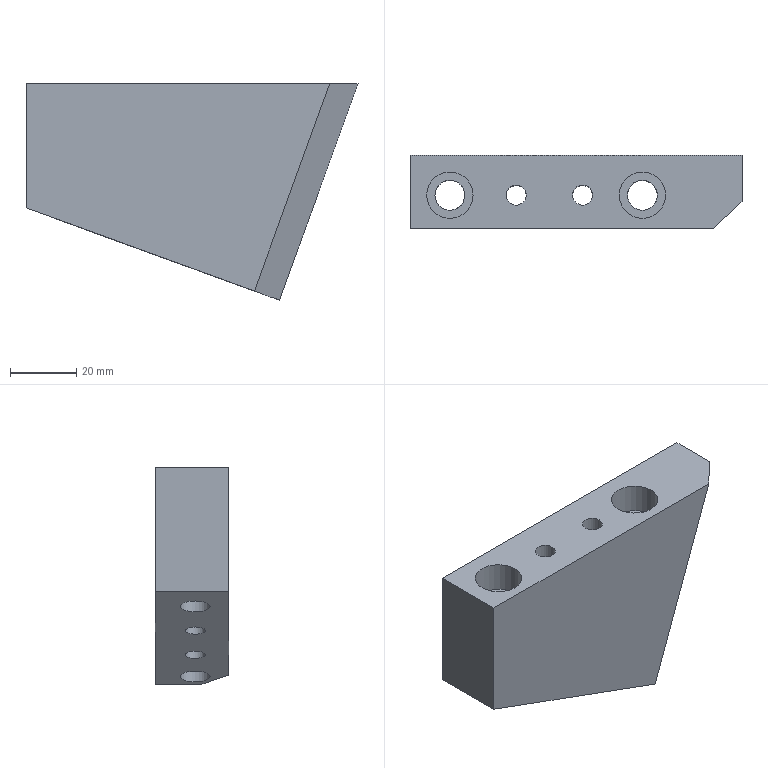Part | STEP file | P011002S002-005 | 1 solid | 15 faces | box 100 x 22 x 65.128 mm | volume 89552 mm3 | plane 9 | cylinder 6 | commonest cylinder face diameters 6 x2 9 x2 14 x2
STEP:
#1=CARTESIAN_POINT('',(0.,0.,0.));
#2=DIRECTION('',(0.,0.,1.));
#3=DIRECTION('',(1.,0.,0.));
#4=AXIS2_PLACEMENT_3D('',#1,#2,#3);
#5=CARTESIAN_POINT('',(194.,-102.,19.));
#6=VERTEX_POINT('',#5);
#7=CARTESIAN_POINT('',(200.,-102.,19.));
#8=VERTEX_POINT('',#7);
#9=CARTESIAN_POINT('',(197.,-102.,19.));
#10=DIRECTION('',(0.,0.,-1.));
#11=DIRECTION('',(-1.,0.,0.));
#12=AXIS2_PLACEMENT_3D('',#9,#10,#11);
#13=CIRCLE('',#12,3.);
#14=CARTESIAN_POINT('',(-275.,-277.,19.));
#15=DIRECTION('',(0.,0.,1.));
#16=DIRECTION('',(-1.,0.,0.));
#17=AXIS2_PLACEMENT_3D('',#14,#15,#16);
#18=PLANE('',#17);
#19=CARTESIAN_POINT('',(-469.,-175.));
#20=CARTESIAN_POINT('',(-469.,-180.196));
#21=CARTESIAN_POINT('',(-473.5,-177.598));
#22=CARTESIAN_POINT('',(-478.,-175.));
#23=CARTESIAN_POINT('',(-473.5,-172.402));
#24=CARTESIAN_POINT('',(-469.,-169.804));
#25=CARTESIAN_POINT('',(-469.,-175.));
#26=(BOUNDED_CURVE()B_SPLINE_CURVE(2,(#19,#20,#21,#22,#23,#24,#25),.UNSPECIFIED.,.T.,.F.)B_SPLINE_CURVE_WITH_KNOTS((1,2,2,2,2,1),(-2.094,0.,2.094,4.189,6.283,8.378),.UNSPECIFIED.)CURVE()GEOMETRIC_REPRESENTATION_ITEM()RATIONAL_B_SPLINE_CURVE((1.,0.5,1.,0.5,1.,0.5,1.))REPRESENTATION_ITEM(''));
#27=(GEOMETRIC_REPRESENTATION_CONTEXT(2)PARAMETRIC_REPRESENTATION_CONTEXT()REPRESENTATION_CONTEXT('',''));
#28=DEFINITIONAL_REPRESENTATION('',(#26),#27);
#29=PCURVE('',#18,#28);
#30=CARTESIAN_POINT('',(197.,-102.,19.));
#31=DIRECTION('',(0.,0.,-1.));
#32=DIRECTION('',(1.,0.,0.));
#33=AXIS2_PLACEMENT_3D('',#30,#31,#32);
#34=CYLINDRICAL_SURFACE('',#33,3.);
#35=CARTESIAN_POINT('',(3.142,0.));
#36=DIRECTION('',(1.,0.));
#37=VECTOR('',#36,1.);
#38=LINE('',#35,#37);
#39=(GEOMETRIC_REPRESENTATION_CONTEXT(2)PARAMETRIC_REPRESENTATION_CONTEXT()REPRESENTATION_CONTEXT('',''));
#40=DEFINITIONAL_REPRESENTATION('',(#38),#39);
#41=PCURVE('',#34,#40);
#42=SURFACE_CURVE('',#13,(#29,#41),.PCURVE_S1.);
#43=EDGE_CURVE('',#6,#8,#42,.T.);
#44=ORIENTED_EDGE('',*,*,#43,.T.);
#45=CARTESIAN_POINT('',(197.,-102.,19.));
#46=DIRECTION('',(0.,0.,-1.));
#47=DIRECTION('',(-1.,0.,0.));
#48=AXIS2_PLACEMENT_3D('',#45,#46,#47);
#49=CIRCLE('',#48,3.);
#50=CARTESIAN_POINT('',(-469.,-175.));
#51=CARTESIAN_POINT('',(-469.,-180.196));
#52=CARTESIAN_POINT('',(-473.5,-177.598));
#53=CARTESIAN_POINT('',(-478.,-175.));
#54=CARTESIAN_POINT('',(-473.5,-172.402));
#55=CARTESIAN_POINT('',(-469.,-169.804));
#56=CARTESIAN_POINT('',(-469.,-175.));
#57=(BOUNDED_CURVE()B_SPLINE_CURVE(2,(#50,#51,#52,#53,#54,#55,#56),.UNSPECIFIED.,.T.,.F.)B_SPLINE_CURVE_WITH_KNOTS((1,2,2,2,2,1),(-2.094,0.,2.094,4.189,6.283,8.378),.UNSPECIFIED.)CURVE()GEOMETRIC_REPRESENTATION_ITEM()RATIONAL_B_SPLINE_CURVE((1.,0.5,1.,0.5,1.,0.5,1.))REPRESENTATION_ITEM(''));
#58=(GEOMETRIC_REPRESENTATION_CONTEXT(2)PARAMETRIC_REPRESENTATION_CONTEXT()REPRESENTATION_CONTEXT('',''));
#59=DEFINITIONAL_REPRESENTATION('',(#57),#58);
#60=PCURVE('',#18,#59);
#61=CARTESIAN_POINT('',(-3.142,0.));
#62=DIRECTION('',(1.,0.));
#63=VECTOR('',#62,1.);
#64=LINE('',#61,#63);
#65=(GEOMETRIC_REPRESENTATION_CONTEXT(2)PARAMETRIC_REPRESENTATION_CONTEXT()REPRESENTATION_CONTEXT('',''));
#66=DEFINITIONAL_REPRESENTATION('',(#64),#65);
#67=PCURVE('',#34,#66);
#68=SURFACE_CURVE('',#49,(#60,#67),.PCURVE_S1.);
#69=EDGE_CURVE('',#8,#6,#68,.T.);
#70=ORIENTED_EDGE('',*,*,#69,.T.);
#71=EDGE_LOOP('',(#44,#70));
#72=FACE_BOUND('',#71,.T.);
#73=CARTESIAN_POINT('',(214.,-102.,19.));
#74=VERTEX_POINT('',#73);
#75=CARTESIAN_POINT('',(220.,-102.,19.));
#76=VERTEX_POINT('',#75);
#77=CARTESIAN_POINT('',(217.,-102.,19.));
#78=DIRECTION('',(0.,0.,-1.));
#79=DIRECTION('',(-1.,0.,0.));
#80=AXIS2_PLACEMENT_3D('',#77,#78,#79);
#81=CIRCLE('',#80,3.);
#82=CARTESIAN_POINT('',(-489.,-175.));
#83=CARTESIAN_POINT('',(-489.,-180.196));
#84=CARTESIAN_POINT('',(-493.5,-177.598));
#85=CARTESIAN_POINT('',(-498.,-175.));
#86=CARTESIAN_POINT('',(-493.5,-172.402));
#87=CARTESIAN_POINT('',(-489.,-169.804));
#88=CARTESIAN_POINT('',(-489.,-175.));
#89=(BOUNDED_CURVE()B_SPLINE_CURVE(2,(#82,#83,#84,#85,#86,#87,#88),.UNSPECIFIED.,.T.,.F.)B_SPLINE_CURVE_WITH_KNOTS((1,2,2,2,2,1),(-2.094,0.,2.094,4.189,6.283,8.378),.UNSPECIFIED.)CURVE()GEOMETRIC_REPRESENTATION_ITEM()RATIONAL_B_SPLINE_CURVE((1.,0.5,1.,0.5,1.,0.5,1.))REPRESENTATION_ITEM(''));
#90=(GEOMETRIC_REPRESENTATION_CONTEXT(2)PARAMETRIC_REPRESENTATION_CONTEXT()REPRESENTATION_CONTEXT('',''));
#91=DEFINITIONAL_REPRESENTATION('',(#89),#90);
#92=PCURVE('',#18,#91);
#93=CARTESIAN_POINT('',(217.,-102.,19.));
#94=DIRECTION('',(0.,0.,-1.));
#95=DIRECTION('',(1.,0.,0.));
#96=AXIS2_PLACEMENT_3D('',#93,#94,#95);
#97=CYLINDRICAL_SURFACE('',#96,3.);
#98=CARTESIAN_POINT('',(3.142,0.));
#99=DIRECTION('',(1.,0.));
#100=VECTOR('',#99,1.);
#101=LINE('',#98,#100);
#102=(GEOMETRIC_REPRESENTATION_CONTEXT(2)PARAMETRIC_REPRESENTATION_CONTEXT()REPRESENTATION_CONTEXT('',''));
#103=DEFINITIONAL_REPRESENTATION('',(#101),#102);
#104=PCURVE('',#97,#103);
#105=SURFACE_CURVE('',#81,(#92,#104),.PCURVE_S1.);
#106=EDGE_CURVE('',#74,#76,#105,.T.);
#107=ORIENTED_EDGE('',*,*,#106,.T.);
#108=CARTESIAN_POINT('',(217.,-102.,19.));
#109=DIRECTION('',(0.,0.,-1.));
#110=DIRECTION('',(-1.,0.,0.));
#111=AXIS2_PLACEMENT_3D('',#108,#109,#110);
#112=CIRCLE('',#111,3.);
#113=CARTESIAN_POINT('',(-489.,-175.));
#114=CARTESIAN_POINT('',(-489.,-180.196));
#115=CARTESIAN_POINT('',(-493.5,-177.598));
#116=CARTESIAN_POINT('',(-498.,-175.));
#117=CARTESIAN_POINT('',(-493.5,-172.402));
#118=CARTESIAN_POINT('',(-489.,-169.804));
#119=CARTESIAN_POINT('',(-489.,-175.));
#120=(BOUNDED_CURVE()B_SPLINE_CURVE(2,(#113,#114,#115,#116,#117,#118,#119),.UNSPECIFIED.,.T.,.F.)B_SPLINE_CURVE_WITH_KNOTS((1,2,2,2,2,1),(-2.094,0.,2.094,4.189,6.283,8.378),.UNSPECIFIED.)CURVE()GEOMETRIC_REPRESENTATION_ITEM()RATIONAL_B_SPLINE_CURVE((1.,0.5,1.,0.5,1.,0.5,1.))REPRESENTATION_ITEM(''));
#121=(GEOMETRIC_REPRESENTATION_CONTEXT(2)PARAMETRIC_REPRESENTATION_CONTEXT()REPRESENTATION_CONTEXT('',''));
#122=DEFINITIONAL_REPRESENTATION('',(#120),#121);
#123=PCURVE('',#18,#122);
#124=CARTESIAN_POINT('',(-3.142,0.));
#125=DIRECTION('',(1.,0.));
#126=VECTOR('',#125,1.);
#127=LINE('',#124,#126);
#128=(GEOMETRIC_REPRESENTATION_CONTEXT(2)PARAMETRIC_REPRESENTATION_CONTEXT()REPRESENTATION_CONTEXT('',''));
#129=DEFINITIONAL_REPRESENTATION('',(#127),#128);
#130=PCURVE('',#97,#129);
#131=SURFACE_CURVE('',#112,(#123,#130),.PCURVE_S1.);
#132=EDGE_CURVE('',#76,#74,#131,.T.);
#133=ORIENTED_EDGE('',*,*,#132,.T.);
#134=EDGE_LOOP('',(#107,#133));
#135=FACE_BOUND('',#134,.T.);
#136=CARTESIAN_POINT('',(265.,-90.,19.));
#137=VERTEX_POINT('',#136);
#138=CARTESIAN_POINT('',(265.,-104.,19.));
#139=VERTEX_POINT('',#138);
#140=CARTESIAN_POINT('',(265.,30.,19.));
#141=DIRECTION('',(0.,-1.,0.));
#142=VECTOR('',#141,1.);
#143=LINE('',#140,#142);
#144=CARTESIAN_POINT('',(-540.,-307.));
#145=DIRECTION('',(0.,1.));
#146=VECTOR('',#145,1.);
#147=LINE('',#144,#146);
#148=(GEOMETRIC_REPRESENTATION_CONTEXT(2)PARAMETRIC_REPRESENTATION_CONTEXT()REPRESENTATION_CONTEXT('',''));
#149=DEFINITIONAL_REPRESENTATION('',(#147),#148);
#150=PCURVE('',#18,#149);
#151=CARTESIAN_POINT('',(265.,30.,19.));
#152=DIRECTION('',(-0.9397,0.,0.342));
#153=DIRECTION('',(-0.342,0.,-0.9397));
#154=AXIS2_PLACEMENT_3D('',#151,#152,#153);
#155=PLANE('',#154);
#156=CARTESIAN_POINT('',(0.,0.));
#157=DIRECTION('',(0.,1.));
#158=VECTOR('',#157,1.);
#159=LINE('',#156,#158);
#160=(GEOMETRIC_REPRESENTATION_CONTEXT(2)PARAMETRIC_REPRESENTATION_CONTEXT()REPRESENTATION_CONTEXT('',''));
#161=DEFINITIONAL_REPRESENTATION('',(#159),#160);
#162=PCURVE('',#155,#161);
#163=SURFACE_CURVE('',#143,(#150,#162),.PCURVE_S1.);
#164=EDGE_CURVE('',#137,#139,#163,.T.);
#165=ORIENTED_EDGE('',*,*,#164,.F.);
#166=CARTESIAN_POINT('',(165.,-90.,19.));
#167=VERTEX_POINT('',#166);
#168=CARTESIAN_POINT('',(227.621,-90.,19.));
#169=DIRECTION('',(-1.,0.,0.));
#170=VECTOR('',#169,1.);
#171=LINE('',#168,#170);
#172=CARTESIAN_POINT('',(-502.621,-187.));
#173=DIRECTION('',(1.,0.));
#174=VECTOR('',#173,1.);
#175=LINE('',#172,#174);
#176=(GEOMETRIC_REPRESENTATION_CONTEXT(2)PARAMETRIC_REPRESENTATION_CONTEXT()REPRESENTATION_CONTEXT('',''));
#177=DEFINITIONAL_REPRESENTATION('',(#175),#176);
#178=PCURVE('',#18,#177);
#179=CARTESIAN_POINT('',(227.621,-90.,-41.15));
#180=DIRECTION('',(0.,1.,0.));
#181=DIRECTION('',(0.,0.,-1.));
#182=AXIS2_PLACEMENT_3D('',#179,#180,#181);
#183=PLANE('',#182);
#184=CARTESIAN_POINT('',(-60.15,0.));
#185=DIRECTION('',(0.,1.));
#186=VECTOR('',#185,1.);
#187=LINE('',#184,#186);
#188=(GEOMETRIC_REPRESENTATION_CONTEXT(2)PARAMETRIC_REPRESENTATION_CONTEXT()REPRESENTATION_CONTEXT('',''));
#189=DEFINITIONAL_REPRESENTATION('',(#187),#188);
#190=PCURVE('',#183,#189);
#191=SURFACE_CURVE('',#171,(#178,#190),.PCURVE_S1.);
#192=EDGE_CURVE('',#137,#167,#191,.T.);
#193=ORIENTED_EDGE('',*,*,#192,.T.);
#194=CARTESIAN_POINT('',(165.,-112.,19.));
#195=VERTEX_POINT('',#194);
#196=CARTESIAN_POINT('',(165.,-277.,19.));
#197=DIRECTION('',(0.,-1.,0.));
#198=VECTOR('',#197,1.);
#199=LINE('',#196,#198);
#200=CARTESIAN_POINT('',(-440.,0.));
#201=DIRECTION('',(0.,1.));
#202=VECTOR('',#201,1.);
#203=LINE('',#200,#202);
#204=(GEOMETRIC_REPRESENTATION_CONTEXT(2)PARAMETRIC_REPRESENTATION_CONTEXT()REPRESENTATION_CONTEXT('',''));
#205=DEFINITIONAL_REPRESENTATION('',(#203),#204);
#206=PCURVE('',#18,#205);
#207=CARTESIAN_POINT('',(165.,30.,0.));
#208=DIRECTION('',(-1.,0.,0.));
#209=DIRECTION('',(0.,0.,-1.));
#210=AXIS2_PLACEMENT_3D('',#207,#208,#209);
#211=PLANE('',#210);
#212=CARTESIAN_POINT('',(-19.,307.));
#213=DIRECTION('',(0.,1.));
#214=VECTOR('',#213,1.);
#215=LINE('',#212,#214);
#216=(GEOMETRIC_REPRESENTATION_CONTEXT(2)PARAMETRIC_REPRESENTATION_CONTEXT()REPRESENTATION_CONTEXT('',''));
#217=DEFINITIONAL_REPRESENTATION('',(#215),#216);
#218=PCURVE('',#211,#217);
#219=SURFACE_CURVE('',#199,(#206,#218),.PCURVE_S1.);
#220=EDGE_CURVE('',#167,#195,#219,.T.);
#221=ORIENTED_EDGE('',*,*,#220,.T.);
#222=CARTESIAN_POINT('',(256.487,-112.,19.));
#223=VERTEX_POINT('',#222);
#224=CARTESIAN_POINT('',(227.621,-112.,19.));
#225=DIRECTION('',(-1.,0.,0.));
#226=VECTOR('',#225,1.);
#227=LINE('',#224,#226);
#228=CARTESIAN_POINT('',(-502.621,-165.));
#229=DIRECTION('',(1.,0.));
#230=VECTOR('',#229,1.);
#231=LINE('',#228,#230);
#232=(GEOMETRIC_REPRESENTATION_CONTEXT(2)PARAMETRIC_REPRESENTATION_CONTEXT()REPRESENTATION_CONTEXT('',''));
#233=DEFINITIONAL_REPRESENTATION('',(#231),#232);
#234=PCURVE('',#18,#233);
#235=CARTESIAN_POINT('',(227.621,-112.,-41.15));
#236=DIRECTION('',(0.,1.,0.));
#237=DIRECTION('',(0.,0.,-1.));
#238=AXIS2_PLACEMENT_3D('',#235,#236,#237);
#239=PLANE('',#238);
#240=CARTESIAN_POINT('',(-60.15,0.));
#241=DIRECTION('',(0.,1.));
#242=VECTOR('',#241,1.);
#243=LINE('',#240,#242);
#244=(GEOMETRIC_REPRESENTATION_CONTEXT(2)PARAMETRIC_REPRESENTATION_CONTEXT()REPRESENTATION_CONTEXT('',''));
#245=DEFINITIONAL_REPRESENTATION('',(#243),#244);
#246=PCURVE('',#239,#245);
#247=SURFACE_CURVE('',#227,(#234,#246),.PCURVE_S1.);
#248=EDGE_CURVE('',#223,#195,#247,.T.);
#249=ORIENTED_EDGE('',*,*,#248,.F.);
#250=CARTESIAN_POINT('',(265.,-104.,19.));
#251=DIRECTION('',(-0.7287,-0.6848,0.));
#252=VECTOR('',#251,1.);
#253=LINE('',#250,#252);
#254=CARTESIAN_POINT('',(-540.,-173.));
#255=DIRECTION('',(0.7287,0.6848));
#256=VECTOR('',#255,1.);
#257=LINE('',#254,#256);
#258=(GEOMETRIC_REPRESENTATION_CONTEXT(2)PARAMETRIC_REPRESENTATION_CONTEXT()REPRESENTATION_CONTEXT('',''));
#259=DEFINITIONAL_REPRESENTATION('',(#257),#258);
#260=PCURVE('',#18,#259);
#261=CARTESIAN_POINT('',(265.,-104.,19.));
#262=DIRECTION('',(-0.6645,0.7071,0.2418));
#263=DIRECTION('',(0.7287,0.6848,0.));
#264=AXIS2_PLACEMENT_3D('',#261,#262,#263);
#265=PLANE('',#264);
#266=CARTESIAN_POINT('',(0.,0.));
#267=DIRECTION('',(-1.,0.));
#268=VECTOR('',#267,1.);
#269=LINE('',#266,#268);
#270=(GEOMETRIC_REPRESENTATION_CONTEXT(2)PARAMETRIC_REPRESENTATION_CONTEXT()REPRESENTATION_CONTEXT('',''));
#271=DEFINITIONAL_REPRESENTATION('',(#269),#270);
#272=PCURVE('',#265,#271);
#273=SURFACE_CURVE('',#253,(#260,#272),.PCURVE_S1.);
#274=EDGE_CURVE('',#139,#223,#273,.T.);
#275=ORIENTED_EDGE('',*,*,#274,.F.);
#276=EDGE_LOOP('',(#165,#193,#221,#249,#275));
#277=FACE_BOUND('',#276,.T.);
#278=CARTESIAN_POINT('',(170.,-102.,19.));
#279=VERTEX_POINT('',#278);
#280=CARTESIAN_POINT('',(177.,-102.,19.));
#281=DIRECTION('',(0.,0.,-1.));
#282=DIRECTION('',(-1.,0.,0.));
#283=AXIS2_PLACEMENT_3D('',#280,#281,#282);
#284=CIRCLE('',#283,7.);
#285=CARTESIAN_POINT('',(-445.,-175.));
#286=CARTESIAN_POINT('',(-445.,-187.124));
#287=CARTESIAN_POINT('',(-455.5,-181.062));
#288=CARTESIAN_POINT('',(-466.,-175.));
#289=CARTESIAN_POINT('',(-455.5,-168.938));
#290=CARTESIAN_POINT('',(-445.,-162.876));
#291=CARTESIAN_POINT('',(-445.,-175.));
#292=(BOUNDED_CURVE()B_SPLINE_CURVE(2,(#285,#286,#287,#288,#289,#290,#291),.UNSPECIFIED.,.T.,.F.)B_SPLINE_CURVE_WITH_KNOTS((1,2,2,2,2,1),(-2.094,0.,2.094,4.189,6.283,8.378),.UNSPECIFIED.)CURVE()GEOMETRIC_REPRESENTATION_ITEM()RATIONAL_B_SPLINE_CURVE((1.,0.5,1.,0.5,1.,0.5,1.))REPRESENTATION_ITEM(''));
#293=(GEOMETRIC_REPRESENTATION_CONTEXT(2)PARAMETRIC_REPRESENTATION_CONTEXT()REPRESENTATION_CONTEXT('',''));
#294=DEFINITIONAL_REPRESENTATION('',(#292),#293);
#295=PCURVE('',#18,#294);
#296=CARTESIAN_POINT('',(177.,-102.,19.));
#297=DIRECTION('',(0.,0.,-1.));
#298=DIRECTION('',(1.,0.,0.));
#299=AXIS2_PLACEMENT_3D('',#296,#297,#298);
#300=CYLINDRICAL_SURFACE('',#299,7.);
#301=CARTESIAN_POINT('',(3.142,0.));
#302=DIRECTION('',(1.,0.));
#303=VECTOR('',#302,1.);
#304=LINE('',#301,#303);
#305=(GEOMETRIC_REPRESENTATION_CONTEXT(2)PARAMETRIC_REPRESENTATION_CONTEXT()REPRESENTATION_CONTEXT('',''));
#306=DEFINITIONAL_REPRESENTATION('',(#304),#305);
#307=PCURVE('',#300,#306);
#308=SURFACE_CURVE('',#284,(#295,#307),.PCURVE_S1.);
#309=EDGE_CURVE('',#279,#279,#308,.T.);
#310=ORIENTED_EDGE('',*,*,#309,.T.);
#311=EDGE_LOOP('',(#310));
#312=FACE_BOUND('',#311,.T.);
#313=CARTESIAN_POINT('',(228.,-102.,19.));
#314=VERTEX_POINT('',#313);
#315=CARTESIAN_POINT('',(235.,-102.,19.));
#316=DIRECTION('',(0.,0.,-1.));
#317=DIRECTION('',(-1.,0.,0.));
#318=AXIS2_PLACEMENT_3D('',#315,#316,#317);
#319=CIRCLE('',#318,7.);
#320=CARTESIAN_POINT('',(-503.,-175.));
#321=CARTESIAN_POINT('',(-503.,-187.124));
#322=CARTESIAN_POINT('',(-513.5,-181.062));
#323=CARTESIAN_POINT('',(-524.,-175.));
#324=CARTESIAN_POINT('',(-513.5,-168.938));
#325=CARTESIAN_POINT('',(-503.,-162.876));
#326=CARTESIAN_POINT('',(-503.,-175.));
#327=(BOUNDED_CURVE()B_SPLINE_CURVE(2,(#320,#321,#322,#323,#324,#325,#326),.UNSPECIFIED.,.T.,.F.)B_SPLINE_CURVE_WITH_KNOTS((1,2,2,2,2,1),(-2.094,0.,2.094,4.189,6.283,8.378),.UNSPECIFIED.)CURVE()GEOMETRIC_REPRESENTATION_ITEM()RATIONAL_B_SPLINE_CURVE((1.,0.5,1.,0.5,1.,0.5,1.))REPRESENTATION_ITEM(''));
#328=(GEOMETRIC_REPRESENTATION_CONTEXT(2)PARAMETRIC_REPRESENTATION_CONTEXT()REPRESENTATION_CONTEXT('',''));
#329=DEFINITIONAL_REPRESENTATION('',(#327),#328);
#330=PCURVE('',#18,#329);
#331=CARTESIAN_POINT('',(235.,-102.,19.));
#332=DIRECTION('',(0.,0.,-1.));
#333=DIRECTION('',(1.,0.,0.));
#334=AXIS2_PLACEMENT_3D('',#331,#332,#333);
#335=CYLINDRICAL_SURFACE('',#334,7.);
#336=CARTESIAN_POINT('',(3.142,0.));
#337=DIRECTION('',(1.,0.));
#338=VECTOR('',#337,1.);
#339=LINE('',#336,#338);
#340=(GEOMETRIC_REPRESENTATION_CONTEXT(2)PARAMETRIC_REPRESENTATION_CONTEXT()REPRESENTATION_CONTEXT('',''));
#341=DEFINITIONAL_REPRESENTATION('',(#339),#340);
#342=PCURVE('',#335,#341);
#343=SURFACE_CURVE('',#319,(#330,#342),.PCURVE_S1.);
#344=EDGE_CURVE('',#314,#314,#343,.T.);
#345=ORIENTED_EDGE('',*,*,#344,.T.);
#346=EDGE_LOOP('',(#345));
#347=FACE_BOUND('',#346,.T.);
#348=ADVANCED_FACE('',(#72,#135,#277,#312,#347),#18,.T.);
#349=CARTESIAN_POINT('',(200.,-102.,-31.097));
#350=VERTEX_POINT('',#349);
#351=CARTESIAN_POINT('',(197.,-102.,-30.005));
#352=DIRECTION('',(0.342,0.,0.9397));
#353=DIRECTION('',(0.9397,0.,-0.342));
#354=AXIS2_PLACEMENT_3D('',#351,#352,#353);
#355=ELLIPSE('',#354,3.193,3.);
#356=CARTESIAN_POINT('',(227.621,-90.,-41.15));
#357=DIRECTION('',(-0.342,0.,-0.9397));
#358=DIRECTION('',(-0.9397,0.,0.342));
#359=AXIS2_PLACEMENT_3D('',#356,#357,#358);
#360=PLANE('',#359);
#361=CARTESIAN_POINT('',(29.393,-12.));
#362=CARTESIAN_POINT('',(29.393,-6.804));
#363=CARTESIAN_POINT('',(34.182,-9.402));
#364=CARTESIAN_POINT('',(38.971,-12.));
#365=CARTESIAN_POINT('',(34.182,-14.598));
#366=CARTESIAN_POINT('',(29.393,-17.196));
#367=CARTESIAN_POINT('',(29.393,-12.));
#368=(BOUNDED_CURVE()B_SPLINE_CURVE(2,(#361,#362,#363,#364,#365,#366,#367),.UNSPECIFIED.,.T.,.F.)B_SPLINE_CURVE_WITH_KNOTS((1,2,2,2,2,1),(-2.094,0.,2.094,4.189,6.283,8.378),.UNSPECIFIED.)CURVE()GEOMETRIC_REPRESENTATION_ITEM()RATIONAL_B_SPLINE_CURVE((1.,0.5,1.,0.5,1.,0.5,1.))REPRESENTATION_ITEM(''));
#369=(GEOMETRIC_REPRESENTATION_CONTEXT(2)PARAMETRIC_REPRESENTATION_CONTEXT()REPRESENTATION_CONTEXT('',''));
#370=DEFINITIONAL_REPRESENTATION('',(#368),#369);
#371=PCURVE('',#360,#370);
#372=CARTESIAN_POINT('',(6.283,50.097));
#373=CARTESIAN_POINT('',(6.188,50.098));
#374=CARTESIAN_POINT('',(5.998,50.067));
#375=CARTESIAN_POINT('',(5.712,49.936));
#376=CARTESIAN_POINT('',(5.426,49.73));
#377=CARTESIAN_POINT('',(5.141,49.465));
#378=CARTESIAN_POINT('',(4.855,49.163));
#379=CARTESIAN_POINT('',(4.57,48.848));
#380=CARTESIAN_POINT('',(4.284,48.545));
#381=CARTESIAN_POINT('',(3.998,48.28));
#382=CARTESIAN_POINT('',(3.713,48.074));
#383=CARTESIAN_POINT('',(3.427,47.943));
#384=CARTESIAN_POINT('',(3.142,47.898));
#385=CARTESIAN_POINT('',(2.856,47.943));
#386=CARTESIAN_POINT('',(2.57,48.074));
#387=CARTESIAN_POINT('',(2.285,48.28));
#388=CARTESIAN_POINT('',(1.999,48.545));
#389=CARTESIAN_POINT('',(1.714,48.848));
#390=CARTESIAN_POINT('',(1.428,49.163));
#391=CARTESIAN_POINT('',(1.142,49.465));
#392=CARTESIAN_POINT('',(0.8568,49.73));
#393=CARTESIAN_POINT('',(0.5712,49.936));
#394=CARTESIAN_POINT('',(0.2856,50.067));
#395=CARTESIAN_POINT('',(0.0952,50.098));
#396=CARTESIAN_POINT('',(0.,50.097));
#397=B_SPLINE_CURVE_WITH_KNOTS('',3,(#372,#373,#374,#375,#376,#377,#378,#379,#380,#381,#382,#383,#384,#385,#386,#387,#388,#389,#390,#391,#392,#393,#394,#395,#396),.UNSPECIFIED.,.F.,.F.,(4,1,1,1,1,1,1,1,1,1,1,1,1,1,1,1,1,1,1,1,1,1,4),(0.,0.2856,0.5712,0.8568,1.142,1.428,1.714,1.999,2.285,2.57,2.856,3.142,3.427,3.713,3.998,4.284,4.57,4.855,5.141,5.426,5.712,5.998,6.283),.QUASI_UNIFORM_KNOTS.);
#398=(GEOMETRIC_REPRESENTATION_CONTEXT(2)PARAMETRIC_REPRESENTATION_CONTEXT()REPRESENTATION_CONTEXT('',''));
#399=DEFINITIONAL_REPRESENTATION('',(#397),#398);
#400=PCURVE('',#34,#399);
#401=SURFACE_CURVE('',#355,(#371,#400),.PCURVE_S1.);
#402=EDGE_CURVE('',#350,#350,#401,.T.);
#403=ORIENTED_EDGE('',*,*,#402,.T.);
#404=EDGE_LOOP('',(#403));
#405=FACE_BOUND('',#404,.T.);
#406=CARTESIAN_POINT('',(220.,-102.,-38.377));
#407=VERTEX_POINT('',#406);
#408=CARTESIAN_POINT('',(217.,-102.,-37.285));
#409=DIRECTION('',(0.342,0.,0.9397));
#410=DIRECTION('',(0.9397,0.,-0.342));
#411=AXIS2_PLACEMENT_3D('',#408,#409,#410);
#412=ELLIPSE('',#411,3.193,3.);
#413=CARTESIAN_POINT('',(8.11,-12.));
#414=CARTESIAN_POINT('',(8.11,-6.804));
#415=CARTESIAN_POINT('',(12.899,-9.402));
#416=CARTESIAN_POINT('',(17.688,-12.));
#417=CARTESIAN_POINT('',(12.899,-14.598));
#418=CARTESIAN_POINT('',(8.11,-17.196));
#419=CARTESIAN_POINT('',(8.11,-12.));
#420=(BOUNDED_CURVE()B_SPLINE_CURVE(2,(#413,#414,#415,#416,#417,#418,#419),.UNSPECIFIED.,.T.,.F.)B_SPLINE_CURVE_WITH_KNOTS((1,2,2,2,2,1),(-2.094,0.,2.094,4.189,6.283,8.378),.UNSPECIFIED.)CURVE()GEOMETRIC_REPRESENTATION_ITEM()RATIONAL_B_SPLINE_CURVE((1.,0.5,1.,0.5,1.,0.5,1.))REPRESENTATION_ITEM(''));
#421=(GEOMETRIC_REPRESENTATION_CONTEXT(2)PARAMETRIC_REPRESENTATION_CONTEXT()REPRESENTATION_CONTEXT('',''));
#422=DEFINITIONAL_REPRESENTATION('',(#420),#421);
#423=PCURVE('',#360,#422);
#424=CARTESIAN_POINT('',(6.283,57.377));
#425=CARTESIAN_POINT('',(6.188,57.377));
#426=CARTESIAN_POINT('',(5.998,57.346));
#427=CARTESIAN_POINT('',(5.712,57.216));
#428=CARTESIAN_POINT('',(5.426,57.009));
#429=CARTESIAN_POINT('',(5.141,56.744));
#430=CARTESIAN_POINT('',(4.855,56.442));
#431=CARTESIAN_POINT('',(4.57,56.127));
#432=CARTESIAN_POINT('',(4.284,55.825));
#433=CARTESIAN_POINT('',(3.998,55.56));
#434=CARTESIAN_POINT('',(3.713,55.354));
#435=CARTESIAN_POINT('',(3.427,55.223));
#436=CARTESIAN_POINT('',(3.142,55.178));
#437=CARTESIAN_POINT('',(2.856,55.223));
#438=CARTESIAN_POINT('',(2.57,55.354));
#439=CARTESIAN_POINT('',(2.285,55.56));
#440=CARTESIAN_POINT('',(1.999,55.825));
#441=CARTESIAN_POINT('',(1.714,56.127));
#442=CARTESIAN_POINT('',(1.428,56.442));
#443=CARTESIAN_POINT('',(1.142,56.744));
#444=CARTESIAN_POINT('',(0.8568,57.009));
#445=CARTESIAN_POINT('',(0.5712,57.216));
#446=CARTESIAN_POINT('',(0.2856,57.346));
#447=CARTESIAN_POINT('',(0.0952,57.377));
#448=CARTESIAN_POINT('',(0.,57.377));
#449=B_SPLINE_CURVE_WITH_KNOTS('',3,(#424,#425,#426,#427,#428,#429,#430,#431,#432,#433,#434,#435,#436,#437,#438,#439,#440,#441,#442,#443,#444,#445,#446,#447,#448),.UNSPECIFIED.,.F.,.F.,(4,1,1,1,1,1,1,1,1,1,1,1,1,1,1,1,1,1,1,1,1,1,4),(0.,0.2856,0.5712,0.8568,1.142,1.428,1.714,1.999,2.285,2.57,2.856,3.142,3.427,3.713,3.998,4.284,4.57,4.855,5.141,5.426,5.712,5.998,6.283),.QUASI_UNIFORM_KNOTS.);
#450=(GEOMETRIC_REPRESENTATION_CONTEXT(2)PARAMETRIC_REPRESENTATION_CONTEXT()REPRESENTATION_CONTEXT('',''));
#451=DEFINITIONAL_REPRESENTATION('',(#449),#450);
#452=PCURVE('',#97,#451);
#453=SURFACE_CURVE('',#412,(#423,#452),.PCURVE_S1.);
#454=EDGE_CURVE('',#407,#407,#453,.T.);
#455=ORIENTED_EDGE('',*,*,#454,.T.);
#456=EDGE_LOOP('',(#455));
#457=FACE_BOUND('',#456,.T.);
#458=CARTESIAN_POINT('',(233.778,-112.,-43.391));
#459=VERTEX_POINT('',#458);
#460=CARTESIAN_POINT('',(165.,-112.,-18.358));
#461=VERTEX_POINT('',#460);
#462=CARTESIAN_POINT('',(227.621,-112.,-41.15));
#463=DIRECTION('',(-0.9397,0.,0.342));
#464=VECTOR('',#463,1.);
#465=LINE('',#462,#464);
#466=CARTESIAN_POINT('',(0.,-22.));
#467=DIRECTION('',(1.,0.));
#468=VECTOR('',#467,1.);
#469=LINE('',#466,#468);
#470=(GEOMETRIC_REPRESENTATION_CONTEXT(2)PARAMETRIC_REPRESENTATION_CONTEXT()REPRESENTATION_CONTEXT('',''));
#471=DEFINITIONAL_REPRESENTATION('',(#469),#470);
#472=PCURVE('',#360,#471);
#473=CARTESIAN_POINT('',(0.,0.));
#474=DIRECTION('',(-0.342,0.9397));
#475=VECTOR('',#474,1.);
#476=LINE('',#473,#475);
#477=(GEOMETRIC_REPRESENTATION_CONTEXT(2)PARAMETRIC_REPRESENTATION_CONTEXT()REPRESENTATION_CONTEXT('',''));
#478=DEFINITIONAL_REPRESENTATION('',(#476),#477);
#479=PCURVE('',#239,#478);
#480=SURFACE_CURVE('',#465,(#472,#479),.PCURVE_S1.);
#481=EDGE_CURVE('',#459,#461,#480,.T.);
#482=ORIENTED_EDGE('',*,*,#481,.T.);
#483=CARTESIAN_POINT('',(165.,-90.,-18.358));
#484=VERTEX_POINT('',#483);
#485=CARTESIAN_POINT('',(165.,30.,-18.358));
#486=DIRECTION('',(0.,-1.,0.));
#487=VECTOR('',#486,1.);
#488=LINE('',#485,#487);
#489=CARTESIAN_POINT('',(66.64,120.));
#490=DIRECTION('',(0.,-1.));
#491=VECTOR('',#490,1.);
#492=LINE('',#489,#491);
#493=(GEOMETRIC_REPRESENTATION_CONTEXT(2)PARAMETRIC_REPRESENTATION_CONTEXT()REPRESENTATION_CONTEXT('',''));
#494=DEFINITIONAL_REPRESENTATION('',(#492),#493);
#495=PCURVE('',#360,#494);
#496=CARTESIAN_POINT('',(18.358,0.));
#497=DIRECTION('',(0.,1.));
#498=VECTOR('',#497,1.);
#499=LINE('',#496,#498);
#500=(GEOMETRIC_REPRESENTATION_CONTEXT(2)PARAMETRIC_REPRESENTATION_CONTEXT()REPRESENTATION_CONTEXT('',''));
#501=DEFINITIONAL_REPRESENTATION('',(#499),#500);
#502=PCURVE('',#211,#501);
#503=SURFACE_CURVE('',#488,(#495,#502),.PCURVE_S1.);
#504=EDGE_CURVE('',#484,#461,#503,.T.);
#505=ORIENTED_EDGE('',*,*,#504,.F.);
#506=CARTESIAN_POINT('',(241.296,-90.,-46.128));
#507=VERTEX_POINT('',#506);
#508=CARTESIAN_POINT('',(227.621,-90.,-41.15));
#509=DIRECTION('',(-0.9397,0.,0.342));
#510=VECTOR('',#509,1.);
#511=LINE('',#508,#510);
#512=CARTESIAN_POINT('',(0.,0.));
#513=DIRECTION('',(1.,0.));
#514=VECTOR('',#513,1.);
#515=LINE('',#512,#514);
#516=(GEOMETRIC_REPRESENTATION_CONTEXT(2)PARAMETRIC_REPRESENTATION_CONTEXT()REPRESENTATION_CONTEXT('',''));
#517=DEFINITIONAL_REPRESENTATION('',(#515),#516);
#518=PCURVE('',#360,#517);
#519=CARTESIAN_POINT('',(0.,0.));
#520=DIRECTION('',(-0.342,0.9397));
#521=VECTOR('',#520,1.);
#522=LINE('',#519,#521);
#523=(GEOMETRIC_REPRESENTATION_CONTEXT(2)PARAMETRIC_REPRESENTATION_CONTEXT()REPRESENTATION_CONTEXT('',''));
#524=DEFINITIONAL_REPRESENTATION('',(#522),#523);
#525=PCURVE('',#183,#524);
#526=SURFACE_CURVE('',#511,(#518,#525),.PCURVE_S1.);
#527=EDGE_CURVE('',#507,#484,#526,.T.);
#528=ORIENTED_EDGE('',*,*,#527,.F.);
#529=CARTESIAN_POINT('',(241.296,-104.,-46.128));
#530=VERTEX_POINT('',#529);
#531=CARTESIAN_POINT('',(241.296,-90.,-46.128));
#532=DIRECTION('',(0.,-1.,0.));
#533=VECTOR('',#532,1.);
#534=LINE('',#531,#533);
#535=CARTESIAN_POINT('',(-14.552,0.));
#536=DIRECTION('',(0.,-1.));
#537=VECTOR('',#536,1.);
#538=LINE('',#535,#537);
#539=(GEOMETRIC_REPRESENTATION_CONTEXT(2)PARAMETRIC_REPRESENTATION_CONTEXT()REPRESENTATION_CONTEXT('',''));
#540=DEFINITIONAL_REPRESENTATION('',(#538),#539);
#541=PCURVE('',#360,#540);
#542=CARTESIAN_POINT('',(69.307,120.));
#543=DIRECTION('',(0.,1.));
#544=VECTOR('',#543,1.);
#545=LINE('',#542,#544);
#546=(GEOMETRIC_REPRESENTATION_CONTEXT(2)PARAMETRIC_REPRESENTATION_CONTEXT()REPRESENTATION_CONTEXT('',''));
#547=DEFINITIONAL_REPRESENTATION('',(#545),#546);
#548=PCURVE('',#155,#547);
#549=SURFACE_CURVE('',#534,(#541,#548),.PCURVE_S1.);
#550=EDGE_CURVE('',#507,#530,#549,.T.);
#551=ORIENTED_EDGE('',*,*,#550,.T.);
#552=CARTESIAN_POINT('',(241.296,-104.,-46.128));
#553=DIRECTION('',(0.6645,0.7071,-0.2418));
#554=VECTOR('',#553,1.);
#555=LINE('',#552,#554);
#556=CARTESIAN_POINT('',(-14.552,-14.));
#557=DIRECTION('',(-0.7071,0.7071));
#558=VECTOR('',#557,1.);
#559=LINE('',#556,#558);
#560=(GEOMETRIC_REPRESENTATION_CONTEXT(2)PARAMETRIC_REPRESENTATION_CONTEXT()REPRESENTATION_CONTEXT('',''));
#561=DEFINITIONAL_REPRESENTATION('',(#559),#560);
#562=PCURVE('',#360,#561);
#563=CARTESIAN_POINT('',(-17.274,67.12));
#564=DIRECTION('',(0.9684,0.2492));
#565=VECTOR('',#564,1.);
#566=LINE('',#563,#565);
#567=(GEOMETRIC_REPRESENTATION_CONTEXT(2)PARAMETRIC_REPRESENTATION_CONTEXT()REPRESENTATION_CONTEXT('',''));
#568=DEFINITIONAL_REPRESENTATION('',(#566),#567);
#569=PCURVE('',#265,#568);
#570=SURFACE_CURVE('',#555,(#562,#569),.PCURVE_S1.);
#571=EDGE_CURVE('',#459,#530,#570,.T.);
#572=ORIENTED_EDGE('',*,*,#571,.F.);
#573=EDGE_LOOP('',(#482,#505,#528,#551,#572));
#574=FACE_BOUND('',#573,.T.);
#575=CARTESIAN_POINT('',(181.5,-102.,-24.364));
#576=VERTEX_POINT('',#575);
#577=CARTESIAN_POINT('',(177.,-102.,-22.726));
#578=DIRECTION('',(0.342,0.,0.9397));
#579=DIRECTION('',(0.9397,0.,-0.342));
#580=AXIS2_PLACEMENT_3D('',#577,#578,#579);
#581=ELLIPSE('',#580,4.789,4.5);
#582=CARTESIAN_POINT('',(49.081,-12.));
#583=CARTESIAN_POINT('',(49.081,-4.206));
#584=CARTESIAN_POINT('',(56.264,-8.103));
#585=CARTESIAN_POINT('',(63.447,-12.));
#586=CARTESIAN_POINT('',(56.264,-15.897));
#587=CARTESIAN_POINT('',(49.081,-19.794));
#588=CARTESIAN_POINT('',(49.081,-12.));
#589=(BOUNDED_CURVE()B_SPLINE_CURVE(2,(#582,#583,#584,#585,#586,#587,#588),.UNSPECIFIED.,.T.,.F.)B_SPLINE_CURVE_WITH_KNOTS((1,2,2,2,2,1),(-2.094,0.,2.094,4.189,6.283,8.378),.UNSPECIFIED.)CURVE()GEOMETRIC_REPRESENTATION_ITEM()RATIONAL_B_SPLINE_CURVE((1.,0.5,1.,0.5,1.,0.5,1.))REPRESENTATION_ITEM(''));
#590=(GEOMETRIC_REPRESENTATION_CONTEXT(2)PARAMETRIC_REPRESENTATION_CONTEXT()REPRESENTATION_CONTEXT('',''));
#591=DEFINITIONAL_REPRESENTATION('',(#589),#590);
#592=PCURVE('',#360,#591);
#593=CARTESIAN_POINT('',(177.,-102.,19.));
#594=DIRECTION('',(0.,0.,-1.));
#595=DIRECTION('',(1.,0.,0.));
#596=AXIS2_PLACEMENT_3D('',#593,#594,#595);
#597=CYLINDRICAL_SURFACE('',#596,4.5);
#598=CARTESIAN_POINT('',(6.283,43.364));
#599=CARTESIAN_POINT('',(6.188,43.365));
#600=CARTESIAN_POINT('',(5.998,43.319));
#601=CARTESIAN_POINT('',(5.712,43.123));
#602=CARTESIAN_POINT('',(5.426,42.813));
#603=CARTESIAN_POINT('',(5.141,42.416));
#604=CARTESIAN_POINT('',(4.855,41.962));
#605=CARTESIAN_POINT('',(4.57,41.49));
#606=CARTESIAN_POINT('',(4.284,41.036));
#607=CARTESIAN_POINT('',(3.998,40.639));
#608=CARTESIAN_POINT('',(3.713,40.329));
#609=CARTESIAN_POINT('',(3.427,40.133));
#610=CARTESIAN_POINT('',(3.142,40.066));
#611=CARTESIAN_POINT('',(2.856,40.133));
#612=CARTESIAN_POINT('',(2.57,40.329));
#613=CARTESIAN_POINT('',(2.285,40.639));
#614=CARTESIAN_POINT('',(1.999,41.036));
#615=CARTESIAN_POINT('',(1.714,41.49));
#616=CARTESIAN_POINT('',(1.428,41.962));
#617=CARTESIAN_POINT('',(1.142,42.416));
#618=CARTESIAN_POINT('',(0.8568,42.813));
#619=CARTESIAN_POINT('',(0.5712,43.123));
#620=CARTESIAN_POINT('',(0.2856,43.319));
#621=CARTESIAN_POINT('',(0.0952,43.365));
#622=CARTESIAN_POINT('',(0.,43.364));
#623=B_SPLINE_CURVE_WITH_KNOTS('',3,(#598,#599,#600,#601,#602,#603,#604,#605,#606,#607,#608,#609,#610,#611,#612,#613,#614,#615,#616,#617,#618,#619,#620,#621,#622),.UNSPECIFIED.,.F.,.F.,(4,1,1,1,1,1,1,1,1,1,1,1,1,1,1,1,1,1,1,1,1,1,4),(0.,0.2856,0.5712,0.8568,1.142,1.428,1.714,1.999,2.285,2.57,2.856,3.142,3.427,3.713,3.998,4.284,4.57,4.855,5.141,5.426,5.712,5.998,6.283),.QUASI_UNIFORM_KNOTS.);
#624=(GEOMETRIC_REPRESENTATION_CONTEXT(2)PARAMETRIC_REPRESENTATION_CONTEXT()REPRESENTATION_CONTEXT('',''));
#625=DEFINITIONAL_REPRESENTATION('',(#623),#624);
#626=PCURVE('',#597,#625);
#627=SURFACE_CURVE('',#581,(#592,#626),.PCURVE_S1.);
#628=EDGE_CURVE('',#576,#576,#627,.T.);
#629=ORIENTED_EDGE('',*,*,#628,.T.);
#630=EDGE_LOOP('',(#629));
#631=FACE_BOUND('',#630,.T.);
#632=CARTESIAN_POINT('',(239.5,-102.,-45.474));
#633=VERTEX_POINT('',#632);
#634=CARTESIAN_POINT('',(235.,-102.,-43.836));
#635=DIRECTION('',(0.342,0.,0.9397));
#636=DIRECTION('',(0.9397,0.,-0.342));
#637=AXIS2_PLACEMENT_3D('',#634,#635,#636);
#638=ELLIPSE('',#637,4.789,4.5);
#639=CARTESIAN_POINT('',(-12.642,-12.));
#640=CARTESIAN_POINT('',(-12.642,-4.206));
#641=CARTESIAN_POINT('',(-5.458,-8.103));
#642=CARTESIAN_POINT('',(1.725,-12.));
#643=CARTESIAN_POINT('',(-5.458,-15.897));
#644=CARTESIAN_POINT('',(-12.642,-19.794));
#645=CARTESIAN_POINT('',(-12.642,-12.));
#646=(BOUNDED_CURVE()B_SPLINE_CURVE(2,(#639,#640,#641,#642,#643,#644,#645),.UNSPECIFIED.,.T.,.F.)B_SPLINE_CURVE_WITH_KNOTS((1,2,2,2,2,1),(-2.094,0.,2.094,4.189,6.283,8.378),.UNSPECIFIED.)CURVE()GEOMETRIC_REPRESENTATION_ITEM()RATIONAL_B_SPLINE_CURVE((1.,0.5,1.,0.5,1.,0.5,1.))REPRESENTATION_ITEM(''));
#647=(GEOMETRIC_REPRESENTATION_CONTEXT(2)PARAMETRIC_REPRESENTATION_CONTEXT()REPRESENTATION_CONTEXT('',''));
#648=DEFINITIONAL_REPRESENTATION('',(#646),#647);
#649=PCURVE('',#360,#648);
#650=CARTESIAN_POINT('',(235.,-102.,19.));
#651=DIRECTION('',(0.,0.,-1.));
#652=DIRECTION('',(1.,0.,0.));
#653=AXIS2_PLACEMENT_3D('',#650,#651,#652);
#654=CYLINDRICAL_SURFACE('',#653,4.5);
#655=CARTESIAN_POINT('',(6.283,64.474));
#656=CARTESIAN_POINT('',(6.188,64.475));
#657=CARTESIAN_POINT('',(5.998,64.429));
#658=CARTESIAN_POINT('',(5.712,64.233));
#659=CARTESIAN_POINT('',(5.426,63.923));
#660=CARTESIAN_POINT('',(5.141,63.526));
#661=CARTESIAN_POINT('',(4.855,63.072));
#662=CARTESIAN_POINT('',(4.57,62.6));
#663=CARTESIAN_POINT('',(4.284,62.146));
#664=CARTESIAN_POINT('',(3.998,61.749));
#665=CARTESIAN_POINT('',(3.713,61.439));
#666=CARTESIAN_POINT('',(3.427,61.243));
#667=CARTESIAN_POINT('',(3.142,61.176));
#668=CARTESIAN_POINT('',(2.856,61.243));
#669=CARTESIAN_POINT('',(2.57,61.439));
#670=CARTESIAN_POINT('',(2.285,61.749));
#671=CARTESIAN_POINT('',(1.999,62.146));
#672=CARTESIAN_POINT('',(1.714,62.6));
#673=CARTESIAN_POINT('',(1.428,63.072));
#674=CARTESIAN_POINT('',(1.142,63.526));
#675=CARTESIAN_POINT('',(0.8568,63.923));
#676=CARTESIAN_POINT('',(0.5712,64.233));
#677=CARTESIAN_POINT('',(0.2856,64.429));
#678=CARTESIAN_POINT('',(0.0952,64.475));
#679=CARTESIAN_POINT('',(0.,64.474));
#680=B_SPLINE_CURVE_WITH_KNOTS('',3,(#655,#656,#657,#658,#659,#660,#661,#662,#663,#664,#665,#666,#667,#668,#669,#670,#671,#672,#673,#674,#675,#676,#677,#678,#679),.UNSPECIFIED.,.F.,.F.,(4,1,1,1,1,1,1,1,1,1,1,1,1,1,1,1,1,1,1,1,1,1,4),(0.,0.2856,0.5712,0.8568,1.142,1.428,1.714,1.999,2.285,2.57,2.856,3.142,3.427,3.713,3.998,4.284,4.57,4.855,5.141,5.426,5.712,5.998,6.283),.QUASI_UNIFORM_KNOTS.);
#681=(GEOMETRIC_REPRESENTATION_CONTEXT(2)PARAMETRIC_REPRESENTATION_CONTEXT()REPRESENTATION_CONTEXT('',''));
#682=DEFINITIONAL_REPRESENTATION('',(#680),#681);
#683=PCURVE('',#654,#682);
#684=SURFACE_CURVE('',#638,(#649,#683),.PCURVE_S1.);
#685=EDGE_CURVE('',#633,#633,#684,.T.);
#686=ORIENTED_EDGE('',*,*,#685,.T.);
#687=EDGE_LOOP('',(#686));
#688=FACE_BOUND('',#687,.T.);
#689=ADVANCED_FACE('',(#405,#457,#574,#631,#688),#360,.T.);
#690=ORIENTED_EDGE('',*,*,#504,.T.);
#691=CARTESIAN_POINT('',(165.,-112.,0.));
#692=DIRECTION('',(0.,0.,1.));
#693=VECTOR('',#692,1.);
#694=LINE('',#691,#693);
#695=CARTESIAN_POINT('',(0.,142.));
#696=DIRECTION('',(-1.,0.));
#697=VECTOR('',#696,1.);
#698=LINE('',#695,#697);
#699=(GEOMETRIC_REPRESENTATION_CONTEXT(2)PARAMETRIC_REPRESENTATION_CONTEXT()REPRESENTATION_CONTEXT('',''));
#700=DEFINITIONAL_REPRESENTATION('',(#698),#699);
#701=PCURVE('',#211,#700);
#702=CARTESIAN_POINT('',(-41.15,62.621));
#703=DIRECTION('',(-1.,0.));
#704=VECTOR('',#703,1.);
#705=LINE('',#702,#704);
#706=(GEOMETRIC_REPRESENTATION_CONTEXT(2)PARAMETRIC_REPRESENTATION_CONTEXT()REPRESENTATION_CONTEXT('',''));
#707=DEFINITIONAL_REPRESENTATION('',(#705),#706);
#708=PCURVE('',#239,#707);
#709=SURFACE_CURVE('',#694,(#701,#708),.PCURVE_S1.);
#710=EDGE_CURVE('',#461,#195,#709,.T.);
#711=ORIENTED_EDGE('',*,*,#710,.T.);
#712=ORIENTED_EDGE('',*,*,#220,.F.);
#713=CARTESIAN_POINT('',(165.,-90.,0.));
#714=DIRECTION('',(0.,0.,1.));
#715=VECTOR('',#714,1.);
#716=LINE('',#713,#715);
#717=CARTESIAN_POINT('',(0.,120.));
#718=DIRECTION('',(-1.,0.));
#719=VECTOR('',#718,1.);
#720=LINE('',#717,#719);
#721=(GEOMETRIC_REPRESENTATION_CONTEXT(2)PARAMETRIC_REPRESENTATION_CONTEXT()REPRESENTATION_CONTEXT('',''));
#722=DEFINITIONAL_REPRESENTATION('',(#720),#721);
#723=PCURVE('',#211,#722);
#724=CARTESIAN_POINT('',(-41.15,62.621));
#725=DIRECTION('',(-1.,0.));
#726=VECTOR('',#725,1.);
#727=LINE('',#724,#726);
#728=(GEOMETRIC_REPRESENTATION_CONTEXT(2)PARAMETRIC_REPRESENTATION_CONTEXT()REPRESENTATION_CONTEXT('',''));
#729=DEFINITIONAL_REPRESENTATION('',(#727),#728);
#730=PCURVE('',#183,#729);
#731=SURFACE_CURVE('',#716,(#723,#730),.PCURVE_S1.);
#732=EDGE_CURVE('',#484,#167,#731,.T.);
#733=ORIENTED_EDGE('',*,*,#732,.F.);
#734=EDGE_LOOP('',(#690,#711,#712,#733));
#735=FACE_BOUND('',#734,.T.);
#736=ADVANCED_FACE('',(#735),#211,.T.);
#737=ORIENTED_EDGE('',*,*,#550,.F.);
#738=CARTESIAN_POINT('',(241.296,-90.,-46.128));
#739=DIRECTION('',(0.342,0.,0.9397));
#740=VECTOR('',#739,1.);
#741=LINE('',#738,#740);
#742=CARTESIAN_POINT('',(69.307,120.));
#743=DIRECTION('',(-1.,0.));
#744=VECTOR('',#743,1.);
#745=LINE('',#742,#744);
#746=(GEOMETRIC_REPRESENTATION_CONTEXT(2)PARAMETRIC_REPRESENTATION_CONTEXT()REPRESENTATION_CONTEXT('',''));
#747=DEFINITIONAL_REPRESENTATION('',(#745),#746);
#748=PCURVE('',#155,#747);
#749=CARTESIAN_POINT('',(4.977,-13.675));
#750=DIRECTION('',(-0.9397,-0.342));
#751=VECTOR('',#750,1.);
#752=LINE('',#749,#751);
#753=(GEOMETRIC_REPRESENTATION_CONTEXT(2)PARAMETRIC_REPRESENTATION_CONTEXT()REPRESENTATION_CONTEXT('',''));
#754=DEFINITIONAL_REPRESENTATION('',(#752),#753);
#755=PCURVE('',#183,#754);
#756=SURFACE_CURVE('',#741,(#748,#755),.PCURVE_S1.);
#757=EDGE_CURVE('',#507,#137,#756,.T.);
#758=ORIENTED_EDGE('',*,*,#757,.T.);
#759=ORIENTED_EDGE('',*,*,#164,.T.);
#760=CARTESIAN_POINT('',(265.,-104.,19.));
#761=DIRECTION('',(0.342,0.,0.9397));
#762=VECTOR('',#761,1.);
#763=LINE('',#760,#762);
#764=CARTESIAN_POINT('',(0.,134.));
#765=DIRECTION('',(-1.,0.));
#766=VECTOR('',#765,1.);
#767=LINE('',#764,#766);
#768=(GEOMETRIC_REPRESENTATION_CONTEXT(2)PARAMETRIC_REPRESENTATION_CONTEXT()REPRESENTATION_CONTEXT('',''));
#769=DEFINITIONAL_REPRESENTATION('',(#767),#768);
#770=PCURVE('',#155,#769);
#771=CARTESIAN_POINT('',(0.,0.));
#772=DIRECTION('',(0.2492,-0.9684));
#773=VECTOR('',#772,1.);
#774=LINE('',#771,#773);
#775=(GEOMETRIC_REPRESENTATION_CONTEXT(2)PARAMETRIC_REPRESENTATION_CONTEXT()REPRESENTATION_CONTEXT('',''));
#776=DEFINITIONAL_REPRESENTATION('',(#774),#775);
#777=PCURVE('',#265,#776);
#778=SURFACE_CURVE('',#763,(#770,#777),.PCURVE_S1.);
#779=EDGE_CURVE('',#530,#139,#778,.T.);
#780=ORIENTED_EDGE('',*,*,#779,.F.);
#781=EDGE_LOOP('',(#737,#758,#759,#780));
#782=FACE_BOUND('',#781,.T.);
#783=ADVANCED_FACE('',(#782),#155,.F.);
#784=ORIENTED_EDGE('',*,*,#248,.T.);
#785=ORIENTED_EDGE('',*,*,#710,.F.);
#786=ORIENTED_EDGE('',*,*,#481,.F.);
#787=CARTESIAN_POINT('',(233.778,-112.,-43.391));
#788=DIRECTION('',(-0.342,0.,-0.9397));
#789=VECTOR('',#788,1.);
#790=LINE('',#787,#789);
#791=CARTESIAN_POINT('',(2.241,-6.157));
#792=DIRECTION('',(0.9397,0.342));
#793=VECTOR('',#792,1.);
#794=LINE('',#791,#793);
#795=(GEOMETRIC_REPRESENTATION_CONTEXT(2)PARAMETRIC_REPRESENTATION_CONTEXT()REPRESENTATION_CONTEXT('',''));
#796=DEFINITIONAL_REPRESENTATION('',(#794),#795);
#797=PCURVE('',#239,#796);
#798=CARTESIAN_POINT('',(-28.231,64.3));
#799=DIRECTION('',(-0.2492,0.9684));
#800=VECTOR('',#799,1.);
#801=LINE('',#798,#800);
#802=(GEOMETRIC_REPRESENTATION_CONTEXT(2)PARAMETRIC_REPRESENTATION_CONTEXT()REPRESENTATION_CONTEXT('',''));
#803=DEFINITIONAL_REPRESENTATION('',(#801),#802);
#804=PCURVE('',#265,#803);
#805=SURFACE_CURVE('',#790,(#797,#804),.PCURVE_S1.);
#806=EDGE_CURVE('',#223,#459,#805,.T.);
#807=ORIENTED_EDGE('',*,*,#806,.F.);
#808=EDGE_LOOP('',(#784,#785,#786,#807));
#809=FACE_BOUND('',#808,.T.);
#810=ADVANCED_FACE('',(#809),#239,.F.);
#811=ORIENTED_EDGE('',*,*,#192,.F.);
#812=ORIENTED_EDGE('',*,*,#757,.F.);
#813=ORIENTED_EDGE('',*,*,#527,.T.);
#814=ORIENTED_EDGE('',*,*,#732,.T.);
#815=EDGE_LOOP('',(#811,#812,#813,#814));
#816=FACE_BOUND('',#815,.T.);
#817=ADVANCED_FACE('',(#816),#183,.T.);
#818=ORIENTED_EDGE('',*,*,#571,.T.);
#819=ORIENTED_EDGE('',*,*,#779,.T.);
#820=ORIENTED_EDGE('',*,*,#274,.T.);
#821=ORIENTED_EDGE('',*,*,#806,.T.);
#822=EDGE_LOOP('',(#818,#819,#820,#821));
#823=FACE_BOUND('',#822,.T.);
#824=ADVANCED_FACE('',(#823),#265,.F.);
#825=ORIENTED_EDGE('',*,*,#106,.T.);
#826=CARTESIAN_POINT('',(220.,-102.,19.));
#827=CARTESIAN_POINT('',(220.,-102.,-38.377));
#828=B_SPLINE_CURVE_WITH_KNOTS('',1,(#826,#827),.UNSPECIFIED.,.F.,.F.,(2,2),(0.,57.377),.PIECEWISE_BEZIER_KNOTS.);
#829=CARTESIAN_POINT('',(6.283,0.));
#830=DIRECTION('',(0.,1.));
#831=VECTOR('',#830,1.);
#832=LINE('',#829,#831);
#833=(GEOMETRIC_REPRESENTATION_CONTEXT(2)PARAMETRIC_REPRESENTATION_CONTEXT()REPRESENTATION_CONTEXT('',''));
#834=DEFINITIONAL_REPRESENTATION('',(#832),#833);
#835=PCURVE('',#97,#834);
#836=CARTESIAN_POINT('',(0.,0.));
#837=DIRECTION('',(0.,1.));
#838=VECTOR('',#837,1.);
#839=LINE('',#836,#838);
#840=(GEOMETRIC_REPRESENTATION_CONTEXT(2)PARAMETRIC_REPRESENTATION_CONTEXT()REPRESENTATION_CONTEXT('',''));
#841=DEFINITIONAL_REPRESENTATION('',(#839),#840);
#842=PCURVE('',#97,#841);
#843=SEAM_CURVE('',#828,(#835,#842),.PCURVE_S1.);
#844=EDGE_CURVE('',#76,#407,#843,.T.);
#845=ORIENTED_EDGE('',*,*,#844,.T.);
#846=ORIENTED_EDGE('',*,*,#454,.T.);
#847=ORIENTED_EDGE('',*,*,#844,.F.);
#848=ORIENTED_EDGE('',*,*,#132,.T.);
#849=EDGE_LOOP('',(#825,#845,#846,#847,#848));
#850=FACE_BOUND('',#849,.F.);
#851=ADVANCED_FACE('',(#850),#97,.F.);
#852=CARTESIAN_POINT('',(172.5,-102.,10.));
#853=VERTEX_POINT('',#852);
#854=CARTESIAN_POINT('',(181.5,-102.,10.));
#855=VERTEX_POINT('',#854);
#856=CARTESIAN_POINT('',(177.,-102.,10.));
#857=DIRECTION('',(0.,0.,-1.));
#858=DIRECTION('',(-1.,0.,0.));
#859=AXIS2_PLACEMENT_3D('',#856,#857,#858);
#860=CIRCLE('',#859,4.5);
#861=CARTESIAN_POINT('',(3.142,9.));
#862=DIRECTION('',(1.,0.));
#863=VECTOR('',#862,1.);
#864=LINE('',#861,#863);
#865=(GEOMETRIC_REPRESENTATION_CONTEXT(2)PARAMETRIC_REPRESENTATION_CONTEXT()REPRESENTATION_CONTEXT('',''));
#866=DEFINITIONAL_REPRESENTATION('',(#864),#865);
#867=PCURVE('',#597,#866);
#868=CARTESIAN_POINT('',(215.,-101.,10.));
#869=DIRECTION('',(0.,0.,1.));
#870=DIRECTION('',(-1.,0.,0.));
#871=AXIS2_PLACEMENT_3D('',#868,#869,#870);
#872=PLANE('',#871);
#873=CARTESIAN_POINT('',(42.5,1.));
#874=CARTESIAN_POINT('',(42.5,-6.794));
#875=CARTESIAN_POINT('',(35.75,-2.897));
#876=CARTESIAN_POINT('',(29.,1.));
#877=CARTESIAN_POINT('',(35.75,4.897));
#878=CARTESIAN_POINT('',(42.5,8.794));
#879=CARTESIAN_POINT('',(42.5,1.));
#880=(BOUNDED_CURVE()B_SPLINE_CURVE(2,(#873,#874,#875,#876,#877,#878,#879),.UNSPECIFIED.,.T.,.F.)B_SPLINE_CURVE_WITH_KNOTS((1,2,2,2,2,1),(-2.094,0.,2.094,4.189,6.283,8.378),.UNSPECIFIED.)CURVE()GEOMETRIC_REPRESENTATION_ITEM()RATIONAL_B_SPLINE_CURVE((1.,0.5,1.,0.5,1.,0.5,1.))REPRESENTATION_ITEM(''));
#881=(GEOMETRIC_REPRESENTATION_CONTEXT(2)PARAMETRIC_REPRESENTATION_CONTEXT()REPRESENTATION_CONTEXT('',''));
#882=DEFINITIONAL_REPRESENTATION('',(#880),#881);
#883=PCURVE('',#872,#882);
#884=SURFACE_CURVE('',#860,(#867,#883),.PCURVE_S1.);
#885=EDGE_CURVE('',#853,#855,#884,.T.);
#886=ORIENTED_EDGE('',*,*,#885,.T.);
#887=CARTESIAN_POINT('',(181.5,-102.,10.));
#888=CARTESIAN_POINT('',(181.5,-102.,-24.364));
#889=B_SPLINE_CURVE_WITH_KNOTS('',1,(#887,#888),.UNSPECIFIED.,.F.,.F.,(2,2),(9.,43.364),.PIECEWISE_BEZIER_KNOTS.);
#890=CARTESIAN_POINT('',(6.283,0.));
#891=DIRECTION('',(0.,1.));
#892=VECTOR('',#891,1.);
#893=LINE('',#890,#892);
#894=(GEOMETRIC_REPRESENTATION_CONTEXT(2)PARAMETRIC_REPRESENTATION_CONTEXT()REPRESENTATION_CONTEXT('',''));
#895=DEFINITIONAL_REPRESENTATION('',(#893),#894);
#896=PCURVE('',#597,#895);
#897=CARTESIAN_POINT('',(0.,0.));
#898=DIRECTION('',(0.,1.));
#899=VECTOR('',#898,1.);
#900=LINE('',#897,#899);
#901=(GEOMETRIC_REPRESENTATION_CONTEXT(2)PARAMETRIC_REPRESENTATION_CONTEXT()REPRESENTATION_CONTEXT('',''));
#902=DEFINITIONAL_REPRESENTATION('',(#900),#901);
#903=PCURVE('',#597,#902);
#904=SEAM_CURVE('',#889,(#896,#903),.PCURVE_S1.);
#905=EDGE_CURVE('',#855,#576,#904,.T.);
#906=ORIENTED_EDGE('',*,*,#905,.T.);
#907=ORIENTED_EDGE('',*,*,#628,.T.);
#908=ORIENTED_EDGE('',*,*,#905,.F.);
#909=CARTESIAN_POINT('',(177.,-102.,10.));
#910=DIRECTION('',(0.,0.,-1.));
#911=DIRECTION('',(-1.,0.,0.));
#912=AXIS2_PLACEMENT_3D('',#909,#910,#911);
#913=CIRCLE('',#912,4.5);
#914=CARTESIAN_POINT('',(-3.142,9.));
#915=DIRECTION('',(1.,0.));
#916=VECTOR('',#915,1.);
#917=LINE('',#914,#916);
#918=(GEOMETRIC_REPRESENTATION_CONTEXT(2)PARAMETRIC_REPRESENTATION_CONTEXT()REPRESENTATION_CONTEXT('',''));
#919=DEFINITIONAL_REPRESENTATION('',(#917),#918);
#920=PCURVE('',#597,#919);
#921=CARTESIAN_POINT('',(42.5,1.));
#922=CARTESIAN_POINT('',(42.5,-6.794));
#923=CARTESIAN_POINT('',(35.75,-2.897));
#924=CARTESIAN_POINT('',(29.,1.));
#925=CARTESIAN_POINT('',(35.75,4.897));
#926=CARTESIAN_POINT('',(42.5,8.794));
#927=CARTESIAN_POINT('',(42.5,1.));
#928=(BOUNDED_CURVE()B_SPLINE_CURVE(2,(#921,#922,#923,#924,#925,#926,#927),.UNSPECIFIED.,.T.,.F.)B_SPLINE_CURVE_WITH_KNOTS((1,2,2,2,2,1),(-2.094,0.,2.094,4.189,6.283,8.378),.UNSPECIFIED.)CURVE()GEOMETRIC_REPRESENTATION_ITEM()RATIONAL_B_SPLINE_CURVE((1.,0.5,1.,0.5,1.,0.5,1.))REPRESENTATION_ITEM(''));
#929=(GEOMETRIC_REPRESENTATION_CONTEXT(2)PARAMETRIC_REPRESENTATION_CONTEXT()REPRESENTATION_CONTEXT('',''));
#930=DEFINITIONAL_REPRESENTATION('',(#928),#929);
#931=PCURVE('',#872,#930);
#932=SURFACE_CURVE('',#913,(#920,#931),.PCURVE_S1.);
#933=EDGE_CURVE('',#855,#853,#932,.T.);
#934=ORIENTED_EDGE('',*,*,#933,.T.);
#935=EDGE_LOOP('',(#886,#906,#907,#908,#934));
#936=FACE_BOUND('',#935,.F.);
#937=ADVANCED_FACE('',(#936),#597,.F.);
#938=CARTESIAN_POINT('',(170.,-102.,10.));
#939=VERTEX_POINT('',#938);
#940=CARTESIAN_POINT('',(177.,-102.,10.));
#941=DIRECTION('',(0.,0.,-1.));
#942=DIRECTION('',(-1.,0.,0.));
#943=AXIS2_PLACEMENT_3D('',#940,#941,#942);
#944=CIRCLE('',#943,7.);
#945=CARTESIAN_POINT('',(45.,1.));
#946=CARTESIAN_POINT('',(45.,-11.124));
#947=CARTESIAN_POINT('',(34.5,-5.062));
#948=CARTESIAN_POINT('',(24.,1.));
#949=CARTESIAN_POINT('',(34.5,7.062));
#950=CARTESIAN_POINT('',(45.,13.124));
#951=CARTESIAN_POINT('',(45.,1.));
#952=(BOUNDED_CURVE()B_SPLINE_CURVE(2,(#945,#946,#947,#948,#949,#950,#951),.UNSPECIFIED.,.T.,.F.)B_SPLINE_CURVE_WITH_KNOTS((1,2,2,2,2,1),(-2.094,0.,2.094,4.189,6.283,8.378),.UNSPECIFIED.)CURVE()GEOMETRIC_REPRESENTATION_ITEM()RATIONAL_B_SPLINE_CURVE((1.,0.5,1.,0.5,1.,0.5,1.))REPRESENTATION_ITEM(''));
#953=(GEOMETRIC_REPRESENTATION_CONTEXT(2)PARAMETRIC_REPRESENTATION_CONTEXT()REPRESENTATION_CONTEXT('',''));
#954=DEFINITIONAL_REPRESENTATION('',(#952),#953);
#955=PCURVE('',#872,#954);
#956=CARTESIAN_POINT('',(3.142,9.));
#957=DIRECTION('',(1.,0.));
#958=VECTOR('',#957,1.);
#959=LINE('',#956,#958);
#960=(GEOMETRIC_REPRESENTATION_CONTEXT(2)PARAMETRIC_REPRESENTATION_CONTEXT()REPRESENTATION_CONTEXT('',''));
#961=DEFINITIONAL_REPRESENTATION('',(#959),#960);
#962=PCURVE('',#300,#961);
#963=SURFACE_CURVE('',#944,(#955,#962),.PCURVE_S1.);
#964=EDGE_CURVE('',#939,#939,#963,.T.);
#965=ORIENTED_EDGE('',*,*,#964,.F.);
#966=EDGE_LOOP('',(#965));
#967=FACE_BOUND('',#966,.T.);
#968=ORIENTED_EDGE('',*,*,#885,.T.);
#969=ORIENTED_EDGE('',*,*,#933,.T.);
#970=EDGE_LOOP('',(#968,#969));
#971=FACE_BOUND('',#970,.T.);
#972=ADVANCED_FACE('',(#967,#971),#872,.T.);
#973=ORIENTED_EDGE('',*,*,#964,.F.);
#974=CARTESIAN_POINT('',(170.,-102.,19.));
#975=CARTESIAN_POINT('',(170.,-102.,10.));
#976=B_SPLINE_CURVE_WITH_KNOTS('',1,(#974,#975),.UNSPECIFIED.,.F.,.F.,(2,2),(0.,9.),.PIECEWISE_BEZIER_KNOTS.);
#977=CARTESIAN_POINT('',(3.142,0.));
#978=DIRECTION('',(0.,1.));
#979=VECTOR('',#978,1.);
#980=LINE('',#977,#979);
#981=(GEOMETRIC_REPRESENTATION_CONTEXT(2)PARAMETRIC_REPRESENTATION_CONTEXT()REPRESENTATION_CONTEXT('',''));
#982=DEFINITIONAL_REPRESENTATION('',(#980),#981);
#983=PCURVE('',#300,#982);
#984=CARTESIAN_POINT('',(9.425,0.));
#985=DIRECTION('',(0.,1.));
#986=VECTOR('',#985,1.);
#987=LINE('',#984,#986);
#988=(GEOMETRIC_REPRESENTATION_CONTEXT(2)PARAMETRIC_REPRESENTATION_CONTEXT()REPRESENTATION_CONTEXT('',''));
#989=DEFINITIONAL_REPRESENTATION('',(#987),#988);
#990=PCURVE('',#300,#989);
#991=SEAM_CURVE('',#976,(#983,#990),.PCURVE_S1.);
#992=EDGE_CURVE('',#279,#939,#991,.T.);
#993=ORIENTED_EDGE('',*,*,#992,.F.);
#994=ORIENTED_EDGE('',*,*,#309,.T.);
#995=ORIENTED_EDGE('',*,*,#992,.T.);
#996=EDGE_LOOP('',(#973,#993,#994,#995));
#997=FACE_BOUND('',#996,.F.);
#998=ADVANCED_FACE('',(#997),#300,.F.);
#999=ORIENTED_EDGE('',*,*,#43,.T.);
#1000=CARTESIAN_POINT('',(200.,-102.,19.));
#1001=CARTESIAN_POINT('',(200.,-102.,-31.097));
#1002=B_SPLINE_CURVE_WITH_KNOTS('',1,(#1000,#1001),.UNSPECIFIED.,.F.,.F.,(2,2),(0.,50.097),.PIECEWISE_BEZIER_KNOTS.);
#1003=CARTESIAN_POINT('',(6.283,0.));
#1004=DIRECTION('',(0.,1.));
#1005=VECTOR('',#1004,1.);
#1006=LINE('',#1003,#1005);
#1007=(GEOMETRIC_REPRESENTATION_CONTEXT(2)PARAMETRIC_REPRESENTATION_CONTEXT()REPRESENTATION_CONTEXT('',''));
#1008=DEFINITIONAL_REPRESENTATION('',(#1006),#1007);
#1009=PCURVE('',#34,#1008);
#1010=CARTESIAN_POINT('',(0.,0.));
#1011=DIRECTION('',(0.,1.));
#1012=VECTOR('',#1011,1.);
#1013=LINE('',#1010,#1012);
#1014=(GEOMETRIC_REPRESENTATION_CONTEXT(2)PARAMETRIC_REPRESENTATION_CONTEXT()REPRESENTATION_CONTEXT('',''));
#1015=DEFINITIONAL_REPRESENTATION('',(#1013),#1014);
#1016=PCURVE('',#34,#1015);
#1017=SEAM_CURVE('',#1002,(#1009,#1016),.PCURVE_S1.);
#1018=EDGE_CURVE('',#8,#350,#1017,.T.);
#1019=ORIENTED_EDGE('',*,*,#1018,.T.);
#1020=ORIENTED_EDGE('',*,*,#402,.T.);
#1021=ORIENTED_EDGE('',*,*,#1018,.F.);
#1022=ORIENTED_EDGE('',*,*,#69,.T.);
#1023=EDGE_LOOP('',(#999,#1019,#1020,#1021,#1022));
#1024=FACE_BOUND('',#1023,.F.);
#1025=ADVANCED_FACE('',(#1024),#34,.F.);
#1026=CARTESIAN_POINT('',(230.5,-102.,10.));
#1027=VERTEX_POINT('',#1026);
#1028=CARTESIAN_POINT('',(239.5,-102.,10.));
#1029=VERTEX_POINT('',#1028);
#1030=CARTESIAN_POINT('',(235.,-102.,10.));
#1031=DIRECTION('',(0.,0.,-1.));
#1032=DIRECTION('',(-1.,0.,0.));
#1033=AXIS2_PLACEMENT_3D('',#1030,#1031,#1032);
#1034=CIRCLE('',#1033,4.5);
#1035=CARTESIAN_POINT('',(3.142,9.));
#1036=DIRECTION('',(1.,0.));
#1037=VECTOR('',#1036,1.);
#1038=LINE('',#1035,#1037);
#1039=(GEOMETRIC_REPRESENTATION_CONTEXT(2)PARAMETRIC_REPRESENTATION_CONTEXT()REPRESENTATION_CONTEXT('',''));
#1040=DEFINITIONAL_REPRESENTATION('',(#1038),#1039);
#1041=PCURVE('',#654,#1040);
#1042=CARTESIAN_POINT('',(215.,-101.,10.));
#1043=DIRECTION('',(0.,0.,1.));
#1044=DIRECTION('',(-1.,0.,0.));
#1045=AXIS2_PLACEMENT_3D('',#1042,#1043,#1044);
#1046=PLANE('',#1045);
#1047=CARTESIAN_POINT('',(-15.5,1.));
#1048=CARTESIAN_POINT('',(-15.5,-6.794));
#1049=CARTESIAN_POINT('',(-22.25,-2.897));
#1050=CARTESIAN_POINT('',(-29.,1.));
#1051=CARTESIAN_POINT('',(-22.25,4.897));
#1052=CARTESIAN_POINT('',(-15.5,8.794));
#1053=CARTESIAN_POINT('',(-15.5,1.));
#1054=(BOUNDED_CURVE()B_SPLINE_CURVE(2,(#1047,#1048,#1049,#1050,#1051,#1052,#1053),.UNSPECIFIED.,.T.,.F.)B_SPLINE_CURVE_WITH_KNOTS((1,2,2,2,2,1),(-2.094,0.,2.094,4.189,6.283,8.378),.UNSPECIFIED.)CURVE()GEOMETRIC_REPRESENTATION_ITEM()RATIONAL_B_SPLINE_CURVE((1.,0.5,1.,0.5,1.,0.5,1.))REPRESENTATION_ITEM(''));
#1055=(GEOMETRIC_REPRESENTATION_CONTEXT(2)PARAMETRIC_REPRESENTATION_CONTEXT()REPRESENTATION_CONTEXT('',''));
#1056=DEFINITIONAL_REPRESENTATION('',(#1054),#1055);
#1057=PCURVE('',#1046,#1056);
#1058=SURFACE_CURVE('',#1034,(#1041,#1057),.PCURVE_S1.);
#1059=EDGE_CURVE('',#1027,#1029,#1058,.T.);
#1060=ORIENTED_EDGE('',*,*,#1059,.T.);
#1061=CARTESIAN_POINT('',(239.5,-102.,10.));
#1062=CARTESIAN_POINT('',(239.5,-102.,-45.474));
#1063=B_SPLINE_CURVE_WITH_KNOTS('',1,(#1061,#1062),.UNSPECIFIED.,.F.,.F.,(2,2),(9.,64.474),.PIECEWISE_BEZIER_KNOTS.);
#1064=CARTESIAN_POINT('',(6.283,0.));
#1065=DIRECTION('',(0.,1.));
#1066=VECTOR('',#1065,1.);
#1067=LINE('',#1064,#1066);
#1068=(GEOMETRIC_REPRESENTATION_CONTEXT(2)PARAMETRIC_REPRESENTATION_CONTEXT()REPRESENTATION_CONTEXT('',''));
#1069=DEFINITIONAL_REPRESENTATION('',(#1067),#1068);
#1070=PCURVE('',#654,#1069);
#1071=CARTESIAN_POINT('',(0.,0.));
#1072=DIRECTION('',(0.,1.));
#1073=VECTOR('',#1072,1.);
#1074=LINE('',#1071,#1073);
#1075=(GEOMETRIC_REPRESENTATION_CONTEXT(2)PARAMETRIC_REPRESENTATION_CONTEXT()REPRESENTATION_CONTEXT('',''));
#1076=DEFINITIONAL_REPRESENTATION('',(#1074),#1075);
#1077=PCURVE('',#654,#1076);
#1078=SEAM_CURVE('',#1063,(#1070,#1077),.PCURVE_S1.);
#1079=EDGE_CURVE('',#1029,#633,#1078,.T.);
#1080=ORIENTED_EDGE('',*,*,#1079,.T.);
#1081=ORIENTED_EDGE('',*,*,#685,.T.);
#1082=ORIENTED_EDGE('',*,*,#1079,.F.);
#1083=CARTESIAN_POINT('',(235.,-102.,10.));
#1084=DIRECTION('',(0.,0.,-1.));
#1085=DIRECTION('',(-1.,0.,0.));
#1086=AXIS2_PLACEMENT_3D('',#1083,#1084,#1085);
#1087=CIRCLE('',#1086,4.5);
#1088=CARTESIAN_POINT('',(-3.142,9.));
#1089=DIRECTION('',(1.,0.));
#1090=VECTOR('',#1089,1.);
#1091=LINE('',#1088,#1090);
#1092=(GEOMETRIC_REPRESENTATION_CONTEXT(2)PARAMETRIC_REPRESENTATION_CONTEXT()REPRESENTATION_CONTEXT('',''));
#1093=DEFINITIONAL_REPRESENTATION('',(#1091),#1092);
#1094=PCURVE('',#654,#1093);
#1095=CARTESIAN_POINT('',(-15.5,1.));
#1096=CARTESIAN_POINT('',(-15.5,-6.794));
#1097=CARTESIAN_POINT('',(-22.25,-2.897));
#1098=CARTESIAN_POINT('',(-29.,1.));
#1099=CARTESIAN_POINT('',(-22.25,4.897));
#1100=CARTESIAN_POINT('',(-15.5,8.794));
#1101=CARTESIAN_POINT('',(-15.5,1.));
#1102=(BOUNDED_CURVE()B_SPLINE_CURVE(2,(#1095,#1096,#1097,#1098,#1099,#1100,#1101),.UNSPECIFIED.,.T.,.F.)B_SPLINE_CURVE_WITH_KNOTS((1,2,2,2,2,1),(-2.094,0.,2.094,4.189,6.283,8.378),.UNSPECIFIED.)CURVE()GEOMETRIC_REPRESENTATION_ITEM()RATIONAL_B_SPLINE_CURVE((1.,0.5,1.,0.5,1.,0.5,1.))REPRESENTATION_ITEM(''));
#1103=(GEOMETRIC_REPRESENTATION_CONTEXT(2)PARAMETRIC_REPRESENTATION_CONTEXT()REPRESENTATION_CONTEXT('',''));
#1104=DEFINITIONAL_REPRESENTATION('',(#1102),#1103);
#1105=PCURVE('',#1046,#1104);
#1106=SURFACE_CURVE('',#1087,(#1094,#1105),.PCURVE_S1.);
#1107=EDGE_CURVE('',#1029,#1027,#1106,.T.);
#1108=ORIENTED_EDGE('',*,*,#1107,.T.);
#1109=EDGE_LOOP('',(#1060,#1080,#1081,#1082,#1108));
#1110=FACE_BOUND('',#1109,.F.);
#1111=ADVANCED_FACE('',(#1110),#654,.F.);
#1112=CARTESIAN_POINT('',(228.,-102.,10.));
#1113=VERTEX_POINT('',#1112);
#1114=CARTESIAN_POINT('',(235.,-102.,10.));
#1115=DIRECTION('',(0.,0.,-1.));
#1116=DIRECTION('',(-1.,0.,0.));
#1117=AXIS2_PLACEMENT_3D('',#1114,#1115,#1116);
#1118=CIRCLE('',#1117,7.);
#1119=CARTESIAN_POINT('',(-13.,1.));
#1120=CARTESIAN_POINT('',(-13.,-11.124));
#1121=CARTESIAN_POINT('',(-23.5,-5.062));
#1122=CARTESIAN_POINT('',(-34.,1.));
#1123=CARTESIAN_POINT('',(-23.5,7.062));
#1124=CARTESIAN_POINT('',(-13.,13.124));
#1125=CARTESIAN_POINT('',(-13.,1.));
#1126=(BOUNDED_CURVE()B_SPLINE_CURVE(2,(#1119,#1120,#1121,#1122,#1123,#1124,#1125),.UNSPECIFIED.,.T.,.F.)B_SPLINE_CURVE_WITH_KNOTS((1,2,2,2,2,1),(-2.094,0.,2.094,4.189,6.283,8.378),.UNSPECIFIED.)CURVE()GEOMETRIC_REPRESENTATION_ITEM()RATIONAL_B_SPLINE_CURVE((1.,0.5,1.,0.5,1.,0.5,1.))REPRESENTATION_ITEM(''));
#1127=(GEOMETRIC_REPRESENTATION_CONTEXT(2)PARAMETRIC_REPRESENTATION_CONTEXT()REPRESENTATION_CONTEXT('',''));
#1128=DEFINITIONAL_REPRESENTATION('',(#1126),#1127);
#1129=PCURVE('',#1046,#1128);
#1130=CARTESIAN_POINT('',(3.142,9.));
#1131=DIRECTION('',(1.,0.));
#1132=VECTOR('',#1131,1.);
#1133=LINE('',#1130,#1132);
#1134=(GEOMETRIC_REPRESENTATION_CONTEXT(2)PARAMETRIC_REPRESENTATION_CONTEXT()REPRESENTATION_CONTEXT('',''));
#1135=DEFINITIONAL_REPRESENTATION('',(#1133),#1134);
#1136=PCURVE('',#335,#1135);
#1137=SURFACE_CURVE('',#1118,(#1129,#1136),.PCURVE_S1.);
#1138=EDGE_CURVE('',#1113,#1113,#1137,.T.);
#1139=ORIENTED_EDGE('',*,*,#1138,.F.);
#1140=EDGE_LOOP('',(#1139));
#1141=FACE_BOUND('',#1140,.T.);
#1142=ORIENTED_EDGE('',*,*,#1059,.T.);
#1143=ORIENTED_EDGE('',*,*,#1107,.T.);
#1144=EDGE_LOOP('',(#1142,#1143));
#1145=FACE_BOUND('',#1144,.T.);
#1146=ADVANCED_FACE('',(#1141,#1145),#1046,.T.);
#1147=ORIENTED_EDGE('',*,*,#1138,.F.);
#1148=CARTESIAN_POINT('',(228.,-102.,19.));
#1149=CARTESIAN_POINT('',(228.,-102.,10.));
#1150=B_SPLINE_CURVE_WITH_KNOTS('',1,(#1148,#1149),.UNSPECIFIED.,.F.,.F.,(2,2),(0.,9.),.PIECEWISE_BEZIER_KNOTS.);
#1151=CARTESIAN_POINT('',(3.142,0.));
#1152=DIRECTION('',(0.,1.));
#1153=VECTOR('',#1152,1.);
#1154=LINE('',#1151,#1153);
#1155=(GEOMETRIC_REPRESENTATION_CONTEXT(2)PARAMETRIC_REPRESENTATION_CONTEXT()REPRESENTATION_CONTEXT('',''));
#1156=DEFINITIONAL_REPRESENTATION('',(#1154),#1155);
#1157=PCURVE('',#335,#1156);
#1158=CARTESIAN_POINT('',(9.425,0.));
#1159=DIRECTION('',(0.,1.));
#1160=VECTOR('',#1159,1.);
#1161=LINE('',#1158,#1160);
#1162=(GEOMETRIC_REPRESENTATION_CONTEXT(2)PARAMETRIC_REPRESENTATION_CONTEXT()REPRESENTATION_CONTEXT('',''));
#1163=DEFINITIONAL_REPRESENTATION('',(#1161),#1162);
#1164=PCURVE('',#335,#1163);
#1165=SEAM_CURVE('',#1150,(#1157,#1164),.PCURVE_S1.);
#1166=EDGE_CURVE('',#314,#1113,#1165,.T.);
#1167=ORIENTED_EDGE('',*,*,#1166,.F.);
#1168=ORIENTED_EDGE('',*,*,#344,.T.);
#1169=ORIENTED_EDGE('',*,*,#1166,.T.);
#1170=EDGE_LOOP('',(#1147,#1167,#1168,#1169));
#1171=FACE_BOUND('',#1170,.F.);
#1172=ADVANCED_FACE('',(#1171),#335,.F.);
#1173=CLOSED_SHELL('',(#348,#689,#736,#783,#810,#817,#824,#851,#937,#972,#998,#1025,#1111,#1146,#1172));
#1174=MANIFOLD_SOLID_BREP('',#1173);
#1175=(LENGTH_UNIT()NAMED_UNIT(*)SI_UNIT(.MILLI.,.METRE.));
#1176=UNCERTAINTY_MEASURE_WITH_UNIT(LENGTH_MEASURE(0.000005),#1175,'','');
#1177=(NAMED_UNIT(*)PLANE_ANGLE_UNIT()SI_UNIT($,.RADIAN.));
#1178=(NAMED_UNIT(*)SI_UNIT($,.STERADIAN.)SOLID_ANGLE_UNIT());
#1179=(GEOMETRIC_REPRESENTATION_CONTEXT(3)GLOBAL_UNCERTAINTY_ASSIGNED_CONTEXT((#1176))GLOBAL_UNIT_ASSIGNED_CONTEXT((#1175,#1177,#1178))REPRESENTATION_CONTEXT('',''));
#1180=ADVANCED_BREP_SHAPE_REPRESENTATION('',(#4,#1174),#1179);